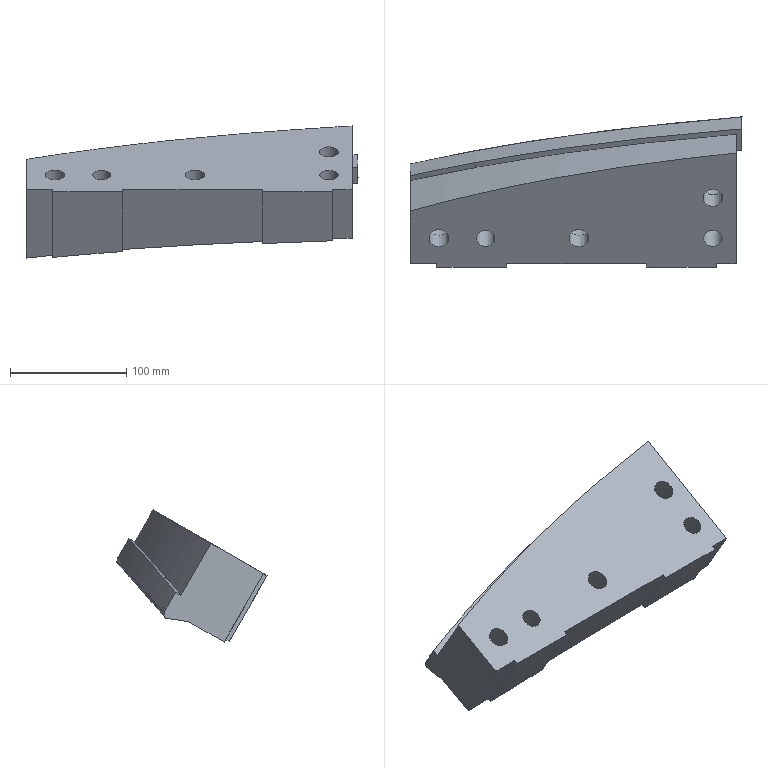Part | NX | features MAIN_BODY 2 | 1 solid | 38 faces | box 285 x 128.929 x 113.4 mm | volume 1293456 mm3 | plane 17 | spline 13 | cylinder 8 | commonest cylinder face diameters 17 x3 26 x3 16 x2